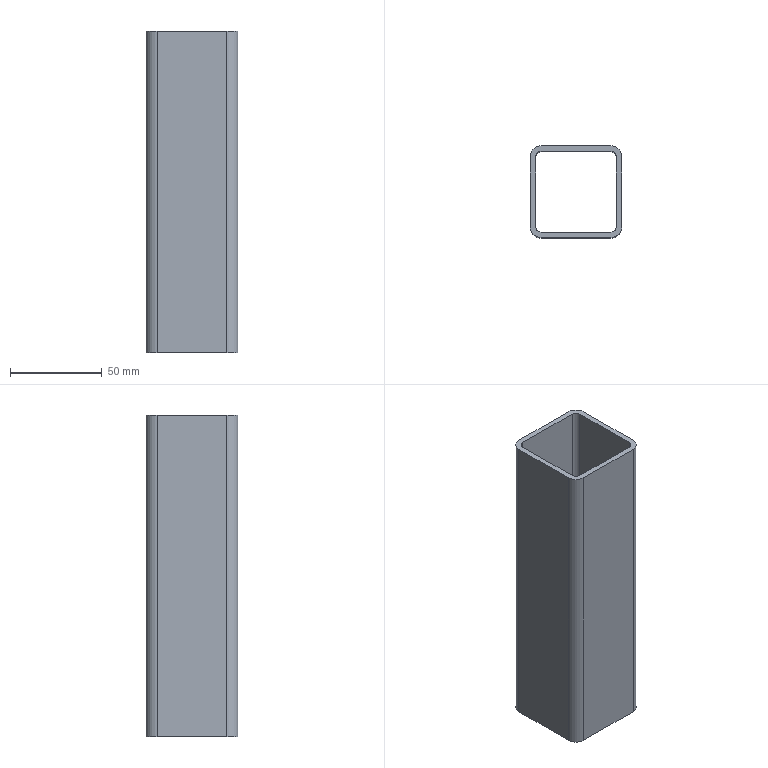Part | SolidWorks | 1 solid | 18 faces | box 50 x 50 x 175 mm | volume 94644 mm3 | plane 10 | cylinder 8 | commonest cylinder face diameters 6 x4 12 x4
STEP:
#1=CARTESIAN_POINT('',(19.,25.,87.5));
#2=VERTEX_POINT('',#1);
#3=CARTESIAN_POINT('',(25.,19.,87.5));
#4=VERTEX_POINT('',#3);
#5=CARTESIAN_POINT('',(19.,19.,87.5));
#6=DIRECTION('',(0.,0.,-1.));
#7=DIRECTION('',(-1.,0.,0.));
#8=AXIS2_PLACEMENT_3D('',#5,#6,#7);
#9=CIRCLE('',#8,6.);
#10=EDGE_CURVE('',#2,#4,#9,.T.);
#11=ORIENTED_EDGE('',*,*,#10,.T.);
#12=CARTESIAN_POINT('',(25.,19.,-87.5));
#13=VERTEX_POINT('',#12);
#14=CARTESIAN_POINT('',(25.,19.,-87.5));
#15=DIRECTION('',(0.,0.,1.));
#16=VECTOR('',#15,1000.);
#17=LINE('',#14,#16);
#18=EDGE_CURVE('',#13,#4,#17,.T.);
#19=ORIENTED_EDGE('',*,*,#18,.F.);
#20=CARTESIAN_POINT('',(19.,25.,-87.5));
#21=VERTEX_POINT('',#20);
#22=CARTESIAN_POINT('',(19.,19.,-87.5));
#23=DIRECTION('',(0.,0.,-1.));
#24=DIRECTION('',(-1.,0.,0.));
#25=AXIS2_PLACEMENT_3D('',#22,#23,#24);
#26=CIRCLE('',#25,6.);
#27=EDGE_CURVE('',#21,#13,#26,.T.);
#28=ORIENTED_EDGE('',*,*,#27,.F.);
#29=CARTESIAN_POINT('',(19.,25.,-87.5));
#30=DIRECTION('',(0.,0.,1.));
#31=VECTOR('',#30,1000.);
#32=LINE('',#29,#31);
#33=EDGE_CURVE('',#21,#2,#32,.T.);
#34=ORIENTED_EDGE('',*,*,#33,.T.);
#35=EDGE_LOOP('',(#11,#19,#28,#34));
#36=FACE_OUTER_BOUND('',#35,.T.);
#37=CARTESIAN_POINT('',(19.,19.,-87.5));
#38=DIRECTION('',(0.,0.,1.));
#39=DIRECTION('',(1.,0.,0.));
#40=AXIS2_PLACEMENT_3D('',#37,#38,#39);
#41=CYLINDRICAL_SURFACE('',#40,6.);
#42=ADVANCED_FACE('',(#36),#41,.T.);
#43=CARTESIAN_POINT('',(25.,-19.,87.5));
#44=VERTEX_POINT('',#43);
#45=CARTESIAN_POINT('',(25.,19.,87.5));
#46=DIRECTION('',(0.,-1.,0.));
#47=VECTOR('',#46,1000.);
#48=LINE('',#45,#47);
#49=EDGE_CURVE('',#4,#44,#48,.T.);
#50=ORIENTED_EDGE('',*,*,#49,.T.);
#51=CARTESIAN_POINT('',(25.,-19.,-87.5));
#52=VERTEX_POINT('',#51);
#53=CARTESIAN_POINT('',(25.,-19.,-87.5));
#54=DIRECTION('',(0.,0.,1.));
#55=VECTOR('',#54,1000.);
#56=LINE('',#53,#55);
#57=EDGE_CURVE('',#52,#44,#56,.T.);
#58=ORIENTED_EDGE('',*,*,#57,.F.);
#59=CARTESIAN_POINT('',(25.,19.,-87.5));
#60=DIRECTION('',(0.,-1.,0.));
#61=VECTOR('',#60,1000.);
#62=LINE('',#59,#61);
#63=EDGE_CURVE('',#13,#52,#62,.T.);
#64=ORIENTED_EDGE('',*,*,#63,.F.);
#65=ORIENTED_EDGE('',*,*,#18,.T.);
#66=EDGE_LOOP('',(#50,#58,#64,#65));
#67=FACE_OUTER_BOUND('',#66,.T.);
#68=CARTESIAN_POINT('',(25.,19.,-87.5));
#69=DIRECTION('',(-1.,0.,0.));
#70=DIRECTION('',(0.,0.,1.));
#71=AXIS2_PLACEMENT_3D('',#68,#69,#70);
#72=PLANE('',#71);
#73=ADVANCED_FACE('',(#67),#72,.F.);
#74=CARTESIAN_POINT('',(19.,-25.,87.5));
#75=VERTEX_POINT('',#74);
#76=CARTESIAN_POINT('',(19.,-19.,87.5));
#77=DIRECTION('',(0.,0.,-1.));
#78=DIRECTION('',(-1.,0.,0.));
#79=AXIS2_PLACEMENT_3D('',#76,#77,#78);
#80=CIRCLE('',#79,6.);
#81=EDGE_CURVE('',#44,#75,#80,.T.);
#82=ORIENTED_EDGE('',*,*,#81,.T.);
#83=CARTESIAN_POINT('',(19.,-25.,-87.5));
#84=VERTEX_POINT('',#83);
#85=CARTESIAN_POINT('',(19.,-25.,-87.5));
#86=DIRECTION('',(0.,0.,1.));
#87=VECTOR('',#86,1000.);
#88=LINE('',#85,#87);
#89=EDGE_CURVE('',#84,#75,#88,.T.);
#90=ORIENTED_EDGE('',*,*,#89,.F.);
#91=CARTESIAN_POINT('',(19.,-19.,-87.5));
#92=DIRECTION('',(0.,0.,-1.));
#93=DIRECTION('',(-1.,0.,0.));
#94=AXIS2_PLACEMENT_3D('',#91,#92,#93);
#95=CIRCLE('',#94,6.);
#96=EDGE_CURVE('',#52,#84,#95,.T.);
#97=ORIENTED_EDGE('',*,*,#96,.F.);
#98=ORIENTED_EDGE('',*,*,#57,.T.);
#99=EDGE_LOOP('',(#82,#90,#97,#98));
#100=FACE_OUTER_BOUND('',#99,.T.);
#101=CARTESIAN_POINT('',(19.,-19.,-87.5));
#102=DIRECTION('',(0.,0.,1.));
#103=DIRECTION('',(1.,0.,0.));
#104=AXIS2_PLACEMENT_3D('',#101,#102,#103);
#105=CYLINDRICAL_SURFACE('',#104,6.);
#106=ADVANCED_FACE('',(#100),#105,.T.);
#107=CARTESIAN_POINT('',(-19.,-25.,87.5));
#108=VERTEX_POINT('',#107);
#109=CARTESIAN_POINT('',(-19.,-25.,87.5));
#110=DIRECTION('',(-1.,0.,0.));
#111=VECTOR('',#110,1000.);
#112=LINE('',#109,#111);
#113=EDGE_CURVE('',#75,#108,#112,.T.);
#114=ORIENTED_EDGE('',*,*,#113,.T.);
#115=CARTESIAN_POINT('',(-19.,-25.,-87.5));
#116=VERTEX_POINT('',#115);
#117=CARTESIAN_POINT('',(-19.,-25.,-87.5));
#118=DIRECTION('',(0.,0.,1.));
#119=VECTOR('',#118,1000.);
#120=LINE('',#117,#119);
#121=EDGE_CURVE('',#116,#108,#120,.T.);
#122=ORIENTED_EDGE('',*,*,#121,.F.);
#123=CARTESIAN_POINT('',(-19.,-25.,-87.5));
#124=DIRECTION('',(-1.,0.,0.));
#125=VECTOR('',#124,1000.);
#126=LINE('',#123,#125);
#127=EDGE_CURVE('',#84,#116,#126,.T.);
#128=ORIENTED_EDGE('',*,*,#127,.F.);
#129=ORIENTED_EDGE('',*,*,#89,.T.);
#130=EDGE_LOOP('',(#114,#122,#128,#129));
#131=FACE_OUTER_BOUND('',#130,.T.);
#132=CARTESIAN_POINT('',(-19.,-25.,-87.5));
#133=DIRECTION('',(0.,1.,0.));
#134=DIRECTION('',(0.,0.,1.));
#135=AXIS2_PLACEMENT_3D('',#132,#133,#134);
#136=PLANE('',#135);
#137=ADVANCED_FACE('',(#131),#136,.F.);
#138=CARTESIAN_POINT('',(-25.,-19.,87.5));
#139=VERTEX_POINT('',#138);
#140=CARTESIAN_POINT('',(-19.,-19.,87.5));
#141=DIRECTION('',(0.,0.,-1.));
#142=DIRECTION('',(-1.,0.,0.));
#143=AXIS2_PLACEMENT_3D('',#140,#141,#142);
#144=CIRCLE('',#143,6.);
#145=EDGE_CURVE('',#108,#139,#144,.T.);
#146=ORIENTED_EDGE('',*,*,#145,.T.);
#147=CARTESIAN_POINT('',(-25.,-19.,-87.5));
#148=VERTEX_POINT('',#147);
#149=CARTESIAN_POINT('',(-25.,-19.,-87.5));
#150=DIRECTION('',(0.,0.,1.));
#151=VECTOR('',#150,1000.);
#152=LINE('',#149,#151);
#153=EDGE_CURVE('',#148,#139,#152,.T.);
#154=ORIENTED_EDGE('',*,*,#153,.F.);
#155=CARTESIAN_POINT('',(-19.,-19.,-87.5));
#156=DIRECTION('',(0.,0.,-1.));
#157=DIRECTION('',(-1.,0.,0.));
#158=AXIS2_PLACEMENT_3D('',#155,#156,#157);
#159=CIRCLE('',#158,6.);
#160=EDGE_CURVE('',#116,#148,#159,.T.);
#161=ORIENTED_EDGE('',*,*,#160,.F.);
#162=ORIENTED_EDGE('',*,*,#121,.T.);
#163=EDGE_LOOP('',(#146,#154,#161,#162));
#164=FACE_OUTER_BOUND('',#163,.T.);
#165=CARTESIAN_POINT('',(-19.,-19.,-87.5));
#166=DIRECTION('',(0.,0.,1.));
#167=DIRECTION('',(1.,0.,0.));
#168=AXIS2_PLACEMENT_3D('',#165,#166,#167);
#169=CYLINDRICAL_SURFACE('',#168,6.);
#170=ADVANCED_FACE('',(#164),#169,.T.);
#171=CARTESIAN_POINT('',(-25.,19.,87.5));
#172=VERTEX_POINT('',#171);
#173=CARTESIAN_POINT('',(-25.,-19.,87.5));
#174=DIRECTION('',(0.,1.,0.));
#175=VECTOR('',#174,1000.);
#176=LINE('',#173,#175);
#177=EDGE_CURVE('',#139,#172,#176,.T.);
#178=ORIENTED_EDGE('',*,*,#177,.T.);
#179=CARTESIAN_POINT('',(-25.,19.,-87.5));
#180=VERTEX_POINT('',#179);
#181=CARTESIAN_POINT('',(-25.,19.,-87.5));
#182=DIRECTION('',(0.,0.,1.));
#183=VECTOR('',#182,1000.);
#184=LINE('',#181,#183);
#185=EDGE_CURVE('',#180,#172,#184,.T.);
#186=ORIENTED_EDGE('',*,*,#185,.F.);
#187=CARTESIAN_POINT('',(-25.,-19.,-87.5));
#188=DIRECTION('',(0.,1.,0.));
#189=VECTOR('',#188,1000.);
#190=LINE('',#187,#189);
#191=EDGE_CURVE('',#148,#180,#190,.T.);
#192=ORIENTED_EDGE('',*,*,#191,.F.);
#193=ORIENTED_EDGE('',*,*,#153,.T.);
#194=EDGE_LOOP('',(#178,#186,#192,#193));
#195=FACE_OUTER_BOUND('',#194,.T.);
#196=CARTESIAN_POINT('',(-25.,-19.,-87.5));
#197=DIRECTION('',(1.,0.,0.));
#198=DIRECTION('',(0.,0.,-1.));
#199=AXIS2_PLACEMENT_3D('',#196,#197,#198);
#200=PLANE('',#199);
#201=ADVANCED_FACE('',(#195),#200,.F.);
#202=CARTESIAN_POINT('',(-19.,25.,87.5));
#203=VERTEX_POINT('',#202);
#204=CARTESIAN_POINT('',(-19.,19.,87.5));
#205=DIRECTION('',(0.,0.,-1.));
#206=DIRECTION('',(-1.,0.,0.));
#207=AXIS2_PLACEMENT_3D('',#204,#205,#206);
#208=CIRCLE('',#207,6.);
#209=EDGE_CURVE('',#172,#203,#208,.T.);
#210=ORIENTED_EDGE('',*,*,#209,.T.);
#211=CARTESIAN_POINT('',(-19.,25.,-87.5));
#212=VERTEX_POINT('',#211);
#213=CARTESIAN_POINT('',(-19.,25.,-87.5));
#214=DIRECTION('',(0.,0.,1.));
#215=VECTOR('',#214,1000.);
#216=LINE('',#213,#215);
#217=EDGE_CURVE('',#212,#203,#216,.T.);
#218=ORIENTED_EDGE('',*,*,#217,.F.);
#219=CARTESIAN_POINT('',(-19.,19.,-87.5));
#220=DIRECTION('',(0.,0.,-1.));
#221=DIRECTION('',(-1.,0.,0.));
#222=AXIS2_PLACEMENT_3D('',#219,#220,#221);
#223=CIRCLE('',#222,6.);
#224=EDGE_CURVE('',#180,#212,#223,.T.);
#225=ORIENTED_EDGE('',*,*,#224,.F.);
#226=ORIENTED_EDGE('',*,*,#185,.T.);
#227=EDGE_LOOP('',(#210,#218,#225,#226));
#228=FACE_OUTER_BOUND('',#227,.T.);
#229=CARTESIAN_POINT('',(-19.,19.,-87.5));
#230=DIRECTION('',(0.,0.,1.));
#231=DIRECTION('',(1.,0.,0.));
#232=AXIS2_PLACEMENT_3D('',#229,#230,#231);
#233=CYLINDRICAL_SURFACE('',#232,6.);
#234=ADVANCED_FACE('',(#228),#233,.T.);
#235=CARTESIAN_POINT('',(22.,-19.,87.5));
#236=VERTEX_POINT('',#235);
#237=CARTESIAN_POINT('',(19.,-22.,87.5));
#238=VERTEX_POINT('',#237);
#239=CARTESIAN_POINT('',(19.,-19.,87.5));
#240=DIRECTION('',(0.,0.,-1.));
#241=DIRECTION('',(-1.,0.,0.));
#242=AXIS2_PLACEMENT_3D('',#239,#240,#241);
#243=CIRCLE('',#242,3.);
#244=EDGE_CURVE('',#236,#238,#243,.T.);
#245=ORIENTED_EDGE('',*,*,#244,.F.);
#246=CARTESIAN_POINT('',(22.,-19.,-87.5));
#247=VERTEX_POINT('',#246);
#248=CARTESIAN_POINT('',(22.,-19.,-87.5));
#249=DIRECTION('',(0.,0.,1.));
#250=VECTOR('',#249,1000.);
#251=LINE('',#248,#250);
#252=EDGE_CURVE('',#247,#236,#251,.T.);
#253=ORIENTED_EDGE('',*,*,#252,.F.);
#254=CARTESIAN_POINT('',(19.,-22.,-87.5));
#255=VERTEX_POINT('',#254);
#256=CARTESIAN_POINT('',(19.,-19.,-87.5));
#257=DIRECTION('',(0.,0.,-1.));
#258=DIRECTION('',(-1.,0.,0.));
#259=AXIS2_PLACEMENT_3D('',#256,#257,#258);
#260=CIRCLE('',#259,3.);
#261=EDGE_CURVE('',#247,#255,#260,.T.);
#262=ORIENTED_EDGE('',*,*,#261,.T.);
#263=CARTESIAN_POINT('',(19.,-22.,-87.5));
#264=DIRECTION('',(0.,0.,1.));
#265=VECTOR('',#264,1000.);
#266=LINE('',#263,#265);
#267=EDGE_CURVE('',#255,#238,#266,.T.);
#268=ORIENTED_EDGE('',*,*,#267,.T.);
#269=EDGE_LOOP('',(#245,#253,#262,#268));
#270=FACE_OUTER_BOUND('',#269,.T.);
#271=CARTESIAN_POINT('',(19.,-19.,-87.5));
#272=DIRECTION('',(0.,0.,1.));
#273=DIRECTION('',(1.,0.,0.));
#274=AXIS2_PLACEMENT_3D('',#271,#272,#273);
#275=CYLINDRICAL_SURFACE('',#274,3.);
#276=ADVANCED_FACE('',(#270),#275,.F.);
#277=CARTESIAN_POINT('',(22.,19.,87.5));
#278=VERTEX_POINT('',#277);
#279=CARTESIAN_POINT('',(22.,19.,87.5));
#280=DIRECTION('',(0.,-1.,0.));
#281=VECTOR('',#280,1000.);
#282=LINE('',#279,#281);
#283=EDGE_CURVE('',#278,#236,#282,.T.);
#284=ORIENTED_EDGE('',*,*,#283,.F.);
#285=CARTESIAN_POINT('',(22.,19.,-87.5));
#286=VERTEX_POINT('',#285);
#287=CARTESIAN_POINT('',(22.,19.,-87.5));
#288=DIRECTION('',(0.,0.,1.));
#289=VECTOR('',#288,1000.);
#290=LINE('',#287,#289);
#291=EDGE_CURVE('',#286,#278,#290,.T.);
#292=ORIENTED_EDGE('',*,*,#291,.F.);
#293=CARTESIAN_POINT('',(22.,19.,-87.5));
#294=DIRECTION('',(0.,-1.,0.));
#295=VECTOR('',#294,1000.);
#296=LINE('',#293,#295);
#297=EDGE_CURVE('',#286,#247,#296,.T.);
#298=ORIENTED_EDGE('',*,*,#297,.T.);
#299=ORIENTED_EDGE('',*,*,#252,.T.);
#300=EDGE_LOOP('',(#284,#292,#298,#299));
#301=FACE_OUTER_BOUND('',#300,.T.);
#302=CARTESIAN_POINT('',(22.,19.,-87.5));
#303=DIRECTION('',(-1.,0.,0.));
#304=DIRECTION('',(0.,0.,1.));
#305=AXIS2_PLACEMENT_3D('',#302,#303,#304);
#306=PLANE('',#305);
#307=ADVANCED_FACE('',(#301),#306,.T.);
#308=CARTESIAN_POINT('',(19.,22.,87.5));
#309=VERTEX_POINT('',#308);
#310=CARTESIAN_POINT('',(19.,19.,87.5));
#311=DIRECTION('',(0.,0.,-1.));
#312=DIRECTION('',(-1.,0.,0.));
#313=AXIS2_PLACEMENT_3D('',#310,#311,#312);
#314=CIRCLE('',#313,3.);
#315=EDGE_CURVE('',#309,#278,#314,.T.);
#316=ORIENTED_EDGE('',*,*,#315,.F.);
#317=CARTESIAN_POINT('',(19.,22.,-87.5));
#318=VERTEX_POINT('',#317);
#319=CARTESIAN_POINT('',(19.,22.,-87.5));
#320=DIRECTION('',(0.,0.,1.));
#321=VECTOR('',#320,1000.);
#322=LINE('',#319,#321);
#323=EDGE_CURVE('',#318,#309,#322,.T.);
#324=ORIENTED_EDGE('',*,*,#323,.F.);
#325=CARTESIAN_POINT('',(19.,19.,-87.5));
#326=DIRECTION('',(0.,0.,-1.));
#327=DIRECTION('',(-1.,0.,0.));
#328=AXIS2_PLACEMENT_3D('',#325,#326,#327);
#329=CIRCLE('',#328,3.);
#330=EDGE_CURVE('',#318,#286,#329,.T.);
#331=ORIENTED_EDGE('',*,*,#330,.T.);
#332=ORIENTED_EDGE('',*,*,#291,.T.);
#333=EDGE_LOOP('',(#316,#324,#331,#332));
#334=FACE_OUTER_BOUND('',#333,.T.);
#335=CARTESIAN_POINT('',(19.,19.,-87.5));
#336=DIRECTION('',(0.,0.,1.));
#337=DIRECTION('',(1.,0.,0.));
#338=AXIS2_PLACEMENT_3D('',#335,#336,#337);
#339=CYLINDRICAL_SURFACE('',#338,3.);
#340=ADVANCED_FACE('',(#334),#339,.F.);
#341=CARTESIAN_POINT('',(-19.,22.,87.5));
#342=VERTEX_POINT('',#341);
#343=CARTESIAN_POINT('',(19.,22.,87.5));
#344=DIRECTION('',(1.,0.,0.));
#345=VECTOR('',#344,1000.);
#346=LINE('',#343,#345);
#347=EDGE_CURVE('',#342,#309,#346,.T.);
#348=ORIENTED_EDGE('',*,*,#347,.F.);
#349=CARTESIAN_POINT('',(-19.,22.,-87.5));
#350=VERTEX_POINT('',#349);
#351=CARTESIAN_POINT('',(-19.,22.,-87.5));
#352=DIRECTION('',(0.,0.,1.));
#353=VECTOR('',#352,1000.);
#354=LINE('',#351,#353);
#355=EDGE_CURVE('',#350,#342,#354,.T.);
#356=ORIENTED_EDGE('',*,*,#355,.F.);
#357=CARTESIAN_POINT('',(19.,22.,-87.5));
#358=DIRECTION('',(1.,0.,0.));
#359=VECTOR('',#358,1000.);
#360=LINE('',#357,#359);
#361=EDGE_CURVE('',#350,#318,#360,.T.);
#362=ORIENTED_EDGE('',*,*,#361,.T.);
#363=ORIENTED_EDGE('',*,*,#323,.T.);
#364=EDGE_LOOP('',(#348,#356,#362,#363));
#365=FACE_OUTER_BOUND('',#364,.T.);
#366=CARTESIAN_POINT('',(19.,22.,-87.5));
#367=DIRECTION('',(0.,-1.,0.));
#368=DIRECTION('',(0.,0.,-1.));
#369=AXIS2_PLACEMENT_3D('',#366,#367,#368);
#370=PLANE('',#369);
#371=ADVANCED_FACE('',(#365),#370,.T.);
#372=CARTESIAN_POINT('',(-22.,19.,87.5));
#373=VERTEX_POINT('',#372);
#374=CARTESIAN_POINT('',(-19.,19.,87.5));
#375=DIRECTION('',(0.,0.,-1.));
#376=DIRECTION('',(-1.,0.,0.));
#377=AXIS2_PLACEMENT_3D('',#374,#375,#376);
#378=CIRCLE('',#377,3.);
#379=EDGE_CURVE('',#373,#342,#378,.T.);
#380=ORIENTED_EDGE('',*,*,#379,.F.);
#381=CARTESIAN_POINT('',(-22.,19.,-87.5));
#382=VERTEX_POINT('',#381);
#383=CARTESIAN_POINT('',(-22.,19.,-87.5));
#384=DIRECTION('',(0.,0.,1.));
#385=VECTOR('',#384,1000.);
#386=LINE('',#383,#385);
#387=EDGE_CURVE('',#382,#373,#386,.T.);
#388=ORIENTED_EDGE('',*,*,#387,.F.);
#389=CARTESIAN_POINT('',(-19.,19.,-87.5));
#390=DIRECTION('',(0.,0.,-1.));
#391=DIRECTION('',(-1.,0.,0.));
#392=AXIS2_PLACEMENT_3D('',#389,#390,#391);
#393=CIRCLE('',#392,3.);
#394=EDGE_CURVE('',#382,#350,#393,.T.);
#395=ORIENTED_EDGE('',*,*,#394,.T.);
#396=ORIENTED_EDGE('',*,*,#355,.T.);
#397=EDGE_LOOP('',(#380,#388,#395,#396));
#398=FACE_OUTER_BOUND('',#397,.T.);
#399=CARTESIAN_POINT('',(-19.,19.,-87.5));
#400=DIRECTION('',(0.,0.,1.));
#401=DIRECTION('',(1.,0.,0.));
#402=AXIS2_PLACEMENT_3D('',#399,#400,#401);
#403=CYLINDRICAL_SURFACE('',#402,3.);
#404=ADVANCED_FACE('',(#398),#403,.F.);
#405=CARTESIAN_POINT('',(-22.,-19.,87.5));
#406=VERTEX_POINT('',#405);
#407=CARTESIAN_POINT('',(-22.,-19.,87.5));
#408=DIRECTION('',(0.,1.,0.));
#409=VECTOR('',#408,1000.);
#410=LINE('',#407,#409);
#411=EDGE_CURVE('',#406,#373,#410,.T.);
#412=ORIENTED_EDGE('',*,*,#411,.F.);
#413=CARTESIAN_POINT('',(-22.,-19.,-87.5));
#414=VERTEX_POINT('',#413);
#415=CARTESIAN_POINT('',(-22.,-19.,-87.5));
#416=DIRECTION('',(0.,0.,1.));
#417=VECTOR('',#416,1000.);
#418=LINE('',#415,#417);
#419=EDGE_CURVE('',#414,#406,#418,.T.);
#420=ORIENTED_EDGE('',*,*,#419,.F.);
#421=CARTESIAN_POINT('',(-22.,-19.,-87.5));
#422=DIRECTION('',(0.,1.,0.));
#423=VECTOR('',#422,1000.);
#424=LINE('',#421,#423);
#425=EDGE_CURVE('',#414,#382,#424,.T.);
#426=ORIENTED_EDGE('',*,*,#425,.T.);
#427=ORIENTED_EDGE('',*,*,#387,.T.);
#428=EDGE_LOOP('',(#412,#420,#426,#427));
#429=FACE_OUTER_BOUND('',#428,.T.);
#430=CARTESIAN_POINT('',(-22.,-19.,-87.5));
#431=DIRECTION('',(1.,0.,0.));
#432=DIRECTION('',(0.,0.,-1.));
#433=AXIS2_PLACEMENT_3D('',#430,#431,#432);
#434=PLANE('',#433);
#435=ADVANCED_FACE('',(#429),#434,.T.);
#436=CARTESIAN_POINT('',(-19.,-22.,87.5));
#437=VERTEX_POINT('',#436);
#438=CARTESIAN_POINT('',(-19.,-19.,87.5));
#439=DIRECTION('',(0.,0.,-1.));
#440=DIRECTION('',(-1.,0.,0.));
#441=AXIS2_PLACEMENT_3D('',#438,#439,#440);
#442=CIRCLE('',#441,3.);
#443=EDGE_CURVE('',#437,#406,#442,.T.);
#444=ORIENTED_EDGE('',*,*,#443,.F.);
#445=CARTESIAN_POINT('',(-19.,-22.,-87.5));
#446=VERTEX_POINT('',#445);
#447=CARTESIAN_POINT('',(-19.,-22.,-87.5));
#448=DIRECTION('',(0.,0.,1.));
#449=VECTOR('',#448,1000.);
#450=LINE('',#447,#449);
#451=EDGE_CURVE('',#446,#437,#450,.T.);
#452=ORIENTED_EDGE('',*,*,#451,.F.);
#453=CARTESIAN_POINT('',(-19.,-19.,-87.5));
#454=DIRECTION('',(0.,0.,-1.));
#455=DIRECTION('',(-1.,0.,0.));
#456=AXIS2_PLACEMENT_3D('',#453,#454,#455);
#457=CIRCLE('',#456,3.);
#458=EDGE_CURVE('',#446,#414,#457,.T.);
#459=ORIENTED_EDGE('',*,*,#458,.T.);
#460=ORIENTED_EDGE('',*,*,#419,.T.);
#461=EDGE_LOOP('',(#444,#452,#459,#460));
#462=FACE_OUTER_BOUND('',#461,.T.);
#463=CARTESIAN_POINT('',(-19.,-19.,-87.5));
#464=DIRECTION('',(0.,0.,1.));
#465=DIRECTION('',(1.,0.,0.));
#466=AXIS2_PLACEMENT_3D('',#463,#464,#465);
#467=CYLINDRICAL_SURFACE('',#466,3.);
#468=ADVANCED_FACE('',(#462),#467,.F.);
#469=CARTESIAN_POINT('',(-19.,-22.,87.5));
#470=DIRECTION('',(-1.,0.,0.));
#471=VECTOR('',#470,1000.);
#472=LINE('',#469,#471);
#473=EDGE_CURVE('',#238,#437,#472,.T.);
#474=ORIENTED_EDGE('',*,*,#473,.F.);
#475=ORIENTED_EDGE('',*,*,#267,.F.);
#476=CARTESIAN_POINT('',(-19.,-22.,-87.5));
#477=DIRECTION('',(-1.,0.,0.));
#478=VECTOR('',#477,1000.);
#479=LINE('',#476,#478);
#480=EDGE_CURVE('',#255,#446,#479,.T.);
#481=ORIENTED_EDGE('',*,*,#480,.T.);
#482=ORIENTED_EDGE('',*,*,#451,.T.);
#483=EDGE_LOOP('',(#474,#475,#481,#482));
#484=FACE_OUTER_BOUND('',#483,.T.);
#485=CARTESIAN_POINT('',(-19.,-22.,-87.5));
#486=DIRECTION('',(0.,1.,0.));
#487=DIRECTION('',(0.,0.,1.));
#488=AXIS2_PLACEMENT_3D('',#485,#486,#487);
#489=PLANE('',#488);
#490=ADVANCED_FACE('',(#484),#489,.T.);
#491=CARTESIAN_POINT('',(19.,25.,87.5));
#492=DIRECTION('',(1.,0.,0.));
#493=VECTOR('',#492,1000.);
#494=LINE('',#491,#493);
#495=EDGE_CURVE('',#203,#2,#494,.T.);
#496=ORIENTED_EDGE('',*,*,#495,.T.);
#497=ORIENTED_EDGE('',*,*,#33,.F.);
#498=CARTESIAN_POINT('',(19.,25.,-87.5));
#499=DIRECTION('',(1.,0.,0.));
#500=VECTOR('',#499,1000.);
#501=LINE('',#498,#500);
#502=EDGE_CURVE('',#212,#21,#501,.T.);
#503=ORIENTED_EDGE('',*,*,#502,.F.);
#504=ORIENTED_EDGE('',*,*,#217,.T.);
#505=EDGE_LOOP('',(#496,#497,#503,#504));
#506=FACE_OUTER_BOUND('',#505,.T.);
#507=CARTESIAN_POINT('',(19.,25.,-87.5));
#508=DIRECTION('',(0.,-1.,0.));
#509=DIRECTION('',(0.,0.,-1.));
#510=AXIS2_PLACEMENT_3D('',#507,#508,#509);
#511=PLANE('',#510);
#512=ADVANCED_FACE('',(#506),#511,.F.);
#513=ORIENTED_EDGE('',*,*,#261,.F.);
#514=ORIENTED_EDGE('',*,*,#297,.F.);
#515=ORIENTED_EDGE('',*,*,#330,.F.);
#516=ORIENTED_EDGE('',*,*,#361,.F.);
#517=ORIENTED_EDGE('',*,*,#394,.F.);
#518=ORIENTED_EDGE('',*,*,#425,.F.);
#519=ORIENTED_EDGE('',*,*,#458,.F.);
#520=ORIENTED_EDGE('',*,*,#480,.F.);
#521=EDGE_LOOP('',(#513,#514,#515,#516,#517,#518,#519,#520));
#522=FACE_BOUND('',#521,.T.);
#523=ORIENTED_EDGE('',*,*,#27,.T.);
#524=ORIENTED_EDGE('',*,*,#63,.T.);
#525=ORIENTED_EDGE('',*,*,#96,.T.);
#526=ORIENTED_EDGE('',*,*,#127,.T.);
#527=ORIENTED_EDGE('',*,*,#160,.T.);
#528=ORIENTED_EDGE('',*,*,#191,.T.);
#529=ORIENTED_EDGE('',*,*,#224,.T.);
#530=ORIENTED_EDGE('',*,*,#502,.T.);
#531=EDGE_LOOP('',(#523,#524,#525,#526,#527,#528,#529,#530));
#532=FACE_OUTER_BOUND('',#531,.T.);
#533=CARTESIAN_POINT('',(19.,19.,-87.5));
#534=DIRECTION('',(0.,0.,-1.));
#535=DIRECTION('',(-1.,0.,0.));
#536=AXIS2_PLACEMENT_3D('',#533,#534,#535);
#537=PLANE('',#536);
#538=ADVANCED_FACE('',(#522,#532),#537,.T.);
#539=ORIENTED_EDGE('',*,*,#244,.T.);
#540=ORIENTED_EDGE('',*,*,#473,.T.);
#541=ORIENTED_EDGE('',*,*,#443,.T.);
#542=ORIENTED_EDGE('',*,*,#411,.T.);
#543=ORIENTED_EDGE('',*,*,#379,.T.);
#544=ORIENTED_EDGE('',*,*,#347,.T.);
#545=ORIENTED_EDGE('',*,*,#315,.T.);
#546=ORIENTED_EDGE('',*,*,#283,.T.);
#547=EDGE_LOOP('',(#539,#540,#541,#542,#543,#544,#545,#546));
#548=FACE_BOUND('',#547,.T.);
#549=ORIENTED_EDGE('',*,*,#10,.F.);
#550=ORIENTED_EDGE('',*,*,#495,.F.);
#551=ORIENTED_EDGE('',*,*,#209,.F.);
#552=ORIENTED_EDGE('',*,*,#177,.F.);
#553=ORIENTED_EDGE('',*,*,#145,.F.);
#554=ORIENTED_EDGE('',*,*,#113,.F.);
#555=ORIENTED_EDGE('',*,*,#81,.F.);
#556=ORIENTED_EDGE('',*,*,#49,.F.);
#557=EDGE_LOOP('',(#549,#550,#551,#552,#553,#554,#555,#556));
#558=FACE_OUTER_BOUND('',#557,.T.);
#559=CARTESIAN_POINT('',(19.,19.,87.5));
#560=DIRECTION('',(0.,0.,-1.));
#561=DIRECTION('',(-1.,0.,0.));
#562=AXIS2_PLACEMENT_3D('',#559,#560,#561);
#563=PLANE('',#562);
#564=ADVANCED_FACE('',(#548,#558),#563,.F.);
#565=CLOSED_SHELL('',(#42,#73,#106,#137,#170,#201,#234,#276,#307,#340,#371,#404,#435,#468,#490,#512,#538,#564));
#566=MANIFOLD_SOLID_BREP('',#565);
#567=CARTESIAN_POINT('',(0.,0.,0.));
#568=DIRECTION('',(0.,0.,1.));
#569=DIRECTION('',(1.,0.,0.));
#570=AXIS2_PLACEMENT_3D('',#567,#568,#569);
#571=(LENGTH_UNIT()NAMED_UNIT(*)SI_UNIT(.MILLI.,.METRE.));
#572=UNCERTAINTY_MEASURE_WITH_UNIT(LENGTH_MEASURE(0.00001),#571,'','');
#573=(NAMED_UNIT(*)PLANE_ANGLE_UNIT()SI_UNIT($,.RADIAN.));
#574=(NAMED_UNIT(*)SI_UNIT($,.STERADIAN.)SOLID_ANGLE_UNIT());
#575=(GEOMETRIC_REPRESENTATION_CONTEXT(3)GLOBAL_UNCERTAINTY_ASSIGNED_CONTEXT((#572))GLOBAL_UNIT_ASSIGNED_CONTEXT((#571,#573,#574))REPRESENTATION_CONTEXT('',''));
#576=ADVANCED_BREP_SHAPE_REPRESENTATION('',(#566,#570),#575);